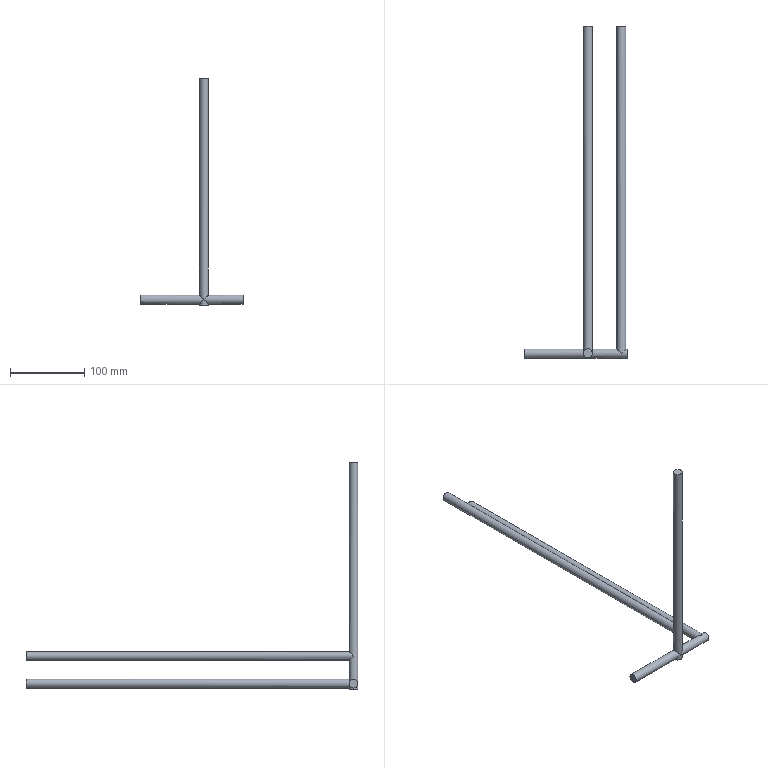Part | STEP file | solid 202 | 1 solid | 12 faces | box 138 x 446 x 305 mm | volume 147324 mm3 | cylinder 6 | plane 6 | commonest cylinder face diameters 12 x6